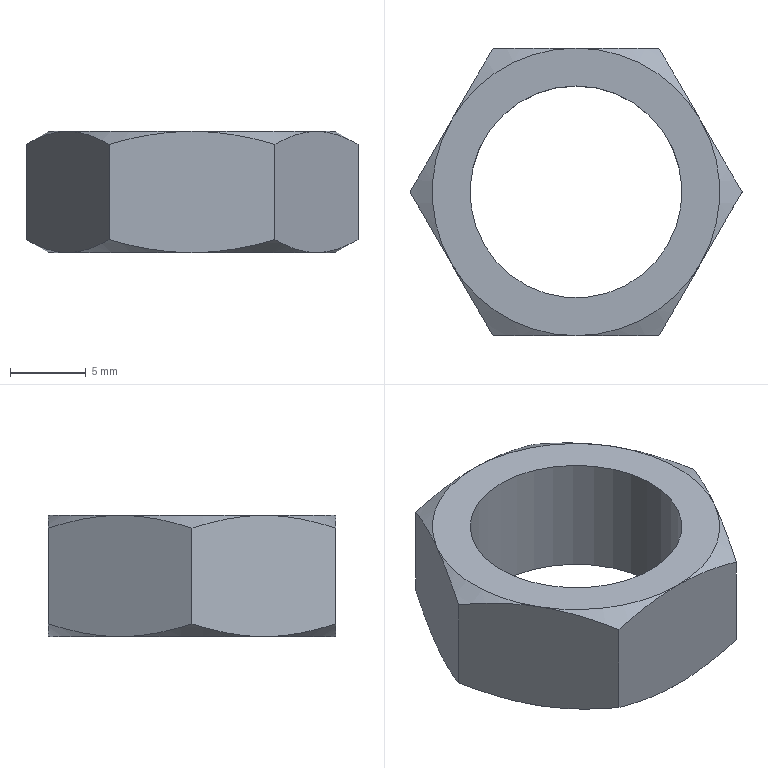Part | STEP file | 冲床-300配套压波_id646_x_t | 1 solid | 21 faces | box 21.939 x 19 x 8 mm | volume 1254 mm3 | cone 12 | plane 8 | cylinder 1 | commonest cylinder face diameters 14 x1
STEP:
#1=CARTESIAN_POINT('',(1810.485,9.5,205.151));
#2=VERTEX_POINT('',#1);
#3=CARTESIAN_POINT('',(1805.,9.5,206.));
#4=VERTEX_POINT('',#3);
#5=CARTESIAN_POINT('',(1810.485,9.5,205.151));
#6=CARTESIAN_POINT('',(1808.693,9.5,205.669));
#7=CARTESIAN_POINT('',(1806.872,9.5,206.));
#8=CARTESIAN_POINT('',(1805.,9.5,206.));
#9=B_SPLINE_CURVE_WITH_KNOTS('',3,(#5,#6,#7,#8),.UNSPECIFIED.,.F.,.F.,(4,4),(0.,1.),.UNSPECIFIED.);
#10=EDGE_CURVE('',#2,#4,#9,.T.);
#11=ORIENTED_EDGE('',*,*,#10,.F.);
#12=CARTESIAN_POINT('',(1810.485,9.5,198.849));
#13=VERTEX_POINT('',#12);
#14=CARTESIAN_POINT('',(1810.485,9.5,198.));
#15=DIRECTION('',(0.,0.,1.));
#16=VECTOR('',#15,1.);
#17=LINE('',#14,#16);
#18=EDGE_CURVE('',#13,#2,#17,.T.);
#19=ORIENTED_EDGE('',*,*,#18,.F.);
#20=CARTESIAN_POINT('',(1805.,9.5,198.));
#21=VERTEX_POINT('',#20);
#22=CARTESIAN_POINT('',(1805.,9.5,198.));
#23=CARTESIAN_POINT('',(1806.872,9.5,198.));
#24=CARTESIAN_POINT('',(1808.693,9.5,198.331));
#25=CARTESIAN_POINT('',(1810.485,9.5,198.849));
#26=B_SPLINE_CURVE_WITH_KNOTS('',3,(#22,#23,#24,#25),.UNSPECIFIED.,.F.,.F.,(4,4),(0.,1.),.UNSPECIFIED.);
#27=EDGE_CURVE('',#21,#13,#26,.T.);
#28=ORIENTED_EDGE('',*,*,#27,.F.);
#29=CARTESIAN_POINT('',(1799.515,9.5,198.849));
#30=VERTEX_POINT('',#29);
#31=CARTESIAN_POINT('',(1799.515,9.5,198.849));
#32=CARTESIAN_POINT('',(1801.307,9.5,198.331));
#33=CARTESIAN_POINT('',(1803.128,9.5,198.));
#34=CARTESIAN_POINT('',(1805.,9.5,198.));
#35=B_SPLINE_CURVE_WITH_KNOTS('',3,(#31,#32,#33,#34),.UNSPECIFIED.,.F.,.F.,(4,4),(0.,1.),.UNSPECIFIED.);
#36=EDGE_CURVE('',#30,#21,#35,.T.);
#37=ORIENTED_EDGE('',*,*,#36,.F.);
#38=CARTESIAN_POINT('',(1799.515,9.5,205.151));
#39=VERTEX_POINT('',#38);
#40=CARTESIAN_POINT('',(1799.515,9.5,198.));
#41=DIRECTION('',(0.,0.,1.));
#42=VECTOR('',#41,1.);
#43=LINE('',#40,#42);
#44=EDGE_CURVE('',#30,#39,#43,.T.);
#45=ORIENTED_EDGE('',*,*,#44,.T.);
#46=CARTESIAN_POINT('',(1805.,9.5,206.));
#47=CARTESIAN_POINT('',(1803.128,9.5,206.));
#48=CARTESIAN_POINT('',(1801.307,9.5,205.669));
#49=CARTESIAN_POINT('',(1799.515,9.5,205.151));
#50=B_SPLINE_CURVE_WITH_KNOTS('',3,(#46,#47,#48,#49),.UNSPECIFIED.,.F.,.F.,(4,4),(0.,1.),.UNSPECIFIED.);
#51=EDGE_CURVE('',#4,#39,#50,.T.);
#52=ORIENTED_EDGE('',*,*,#51,.F.);
#53=EDGE_LOOP('',(#11,#19,#28,#37,#45,#52));
#54=FACE_OUTER_BOUND('',#53,.T.);
#55=CARTESIAN_POINT('',(1799.515,9.5,198.));
#56=DIRECTION('',(0.,-1.,0.));
#57=DIRECTION('',(-1.,0.,0.));
#58=AXIS2_PLACEMENT_3D('',#55,#56,#57);
#59=PLANE('',#58);
#60=ADVANCED_FACE('',(#54),#59,.F.);
#61=CARTESIAN_POINT('',(1815.97,0.,205.151));
#62=VERTEX_POINT('',#61);
#63=CARTESIAN_POINT('',(1813.227,4.75,206.));
#64=VERTEX_POINT('',#63);
#65=CARTESIAN_POINT('',(1815.97,0.,205.151));
#66=CARTESIAN_POINT('',(1815.074,1.552,205.669));
#67=CARTESIAN_POINT('',(1814.163,3.129,206.));
#68=CARTESIAN_POINT('',(1813.227,4.75,206.));
#69=B_SPLINE_CURVE_WITH_KNOTS('',3,(#65,#66,#67,#68),.UNSPECIFIED.,.F.,.F.,(4,4),(0.,1.),.UNSPECIFIED.);
#70=EDGE_CURVE('',#62,#64,#69,.T.);
#71=ORIENTED_EDGE('',*,*,#70,.F.);
#72=CARTESIAN_POINT('',(1815.97,0.,198.849));
#73=VERTEX_POINT('',#72);
#74=CARTESIAN_POINT('',(1815.97,0.,198.));
#75=DIRECTION('',(0.,0.,1.));
#76=VECTOR('',#75,1.);
#77=LINE('',#74,#76);
#78=EDGE_CURVE('',#73,#62,#77,.T.);
#79=ORIENTED_EDGE('',*,*,#78,.F.);
#80=CARTESIAN_POINT('',(1813.227,4.75,198.));
#81=VERTEX_POINT('',#80);
#82=CARTESIAN_POINT('',(1813.227,4.75,198.));
#83=CARTESIAN_POINT('',(1814.163,3.129,198.));
#84=CARTESIAN_POINT('',(1815.074,1.552,198.331));
#85=CARTESIAN_POINT('',(1815.97,0.,198.849));
#86=B_SPLINE_CURVE_WITH_KNOTS('',3,(#82,#83,#84,#85),.UNSPECIFIED.,.F.,.F.,(4,4),(0.,1.),.UNSPECIFIED.);
#87=EDGE_CURVE('',#81,#73,#86,.T.);
#88=ORIENTED_EDGE('',*,*,#87,.F.);
#89=CARTESIAN_POINT('',(1810.485,9.5,198.849));
#90=CARTESIAN_POINT('',(1811.381,7.948,198.331));
#91=CARTESIAN_POINT('',(1812.291,6.371,198.));
#92=CARTESIAN_POINT('',(1813.227,4.75,198.));
#93=B_SPLINE_CURVE_WITH_KNOTS('',3,(#89,#90,#91,#92),.UNSPECIFIED.,.F.,.F.,(4,4),(0.,1.),.UNSPECIFIED.);
#94=EDGE_CURVE('',#13,#81,#93,.T.);
#95=ORIENTED_EDGE('',*,*,#94,.F.);
#96=ORIENTED_EDGE('',*,*,#18,.T.);
#97=CARTESIAN_POINT('',(1813.227,4.75,206.));
#98=CARTESIAN_POINT('',(1812.291,6.371,206.));
#99=CARTESIAN_POINT('',(1811.381,7.948,205.669));
#100=CARTESIAN_POINT('',(1810.485,9.5,205.151));
#101=B_SPLINE_CURVE_WITH_KNOTS('',3,(#97,#98,#99,#100),.UNSPECIFIED.,.F.,.F.,(4,4),(0.,1.),.UNSPECIFIED.);
#102=EDGE_CURVE('',#64,#2,#101,.T.);
#103=ORIENTED_EDGE('',*,*,#102,.F.);
#104=EDGE_LOOP('',(#71,#79,#88,#95,#96,#103));
#105=FACE_OUTER_BOUND('',#104,.T.);
#106=CARTESIAN_POINT('',(1810.485,9.5,198.));
#107=DIRECTION('',(-0.866,-0.5,0.));
#108=DIRECTION('',(-0.5,0.866,0.));
#109=AXIS2_PLACEMENT_3D('',#106,#107,#108);
#110=PLANE('',#109);
#111=ADVANCED_FACE('',(#105),#110,.F.);
#112=CARTESIAN_POINT('',(1810.485,-9.5,205.151));
#113=VERTEX_POINT('',#112);
#114=CARTESIAN_POINT('',(1813.227,-4.75,206.));
#115=VERTEX_POINT('',#114);
#116=CARTESIAN_POINT('',(1810.485,-9.5,205.151));
#117=CARTESIAN_POINT('',(1811.381,-7.948,205.669));
#118=CARTESIAN_POINT('',(1812.291,-6.371,206.));
#119=CARTESIAN_POINT('',(1813.227,-4.75,206.));
#120=B_SPLINE_CURVE_WITH_KNOTS('',3,(#116,#117,#118,#119),.UNSPECIFIED.,.F.,.F.,(4,4),(0.,1.),.UNSPECIFIED.);
#121=EDGE_CURVE('',#113,#115,#120,.T.);
#122=ORIENTED_EDGE('',*,*,#121,.F.);
#123=CARTESIAN_POINT('',(1810.485,-9.5,198.849));
#124=VERTEX_POINT('',#123);
#125=CARTESIAN_POINT('',(1810.485,-9.5,198.));
#126=DIRECTION('',(0.,0.,1.));
#127=VECTOR('',#126,1.);
#128=LINE('',#125,#127);
#129=EDGE_CURVE('',#124,#113,#128,.T.);
#130=ORIENTED_EDGE('',*,*,#129,.F.);
#131=CARTESIAN_POINT('',(1813.227,-4.75,198.));
#132=VERTEX_POINT('',#131);
#133=CARTESIAN_POINT('',(1813.227,-4.75,198.));
#134=CARTESIAN_POINT('',(1812.291,-6.371,198.));
#135=CARTESIAN_POINT('',(1811.381,-7.948,198.331));
#136=CARTESIAN_POINT('',(1810.485,-9.5,198.849));
#137=B_SPLINE_CURVE_WITH_KNOTS('',3,(#133,#134,#135,#136),.UNSPECIFIED.,.F.,.F.,(4,4),(0.,1.),.UNSPECIFIED.);
#138=EDGE_CURVE('',#132,#124,#137,.T.);
#139=ORIENTED_EDGE('',*,*,#138,.F.);
#140=CARTESIAN_POINT('',(1815.97,0.,198.849));
#141=CARTESIAN_POINT('',(1815.074,-1.552,198.331));
#142=CARTESIAN_POINT('',(1814.163,-3.129,198.));
#143=CARTESIAN_POINT('',(1813.227,-4.75,198.));
#144=B_SPLINE_CURVE_WITH_KNOTS('',3,(#140,#141,#142,#143),.UNSPECIFIED.,.F.,.F.,(4,4),(0.,1.),.UNSPECIFIED.);
#145=EDGE_CURVE('',#73,#132,#144,.T.);
#146=ORIENTED_EDGE('',*,*,#145,.F.);
#147=ORIENTED_EDGE('',*,*,#78,.T.);
#148=CARTESIAN_POINT('',(1813.227,-4.75,206.));
#149=CARTESIAN_POINT('',(1814.163,-3.129,206.));
#150=CARTESIAN_POINT('',(1815.074,-1.552,205.669));
#151=CARTESIAN_POINT('',(1815.97,0.,205.151));
#152=B_SPLINE_CURVE_WITH_KNOTS('',3,(#148,#149,#150,#151),.UNSPECIFIED.,.F.,.F.,(4,4),(0.,1.),.UNSPECIFIED.);
#153=EDGE_CURVE('',#115,#62,#152,.T.);
#154=ORIENTED_EDGE('',*,*,#153,.F.);
#155=EDGE_LOOP('',(#122,#130,#139,#146,#147,#154));
#156=FACE_OUTER_BOUND('',#155,.T.);
#157=CARTESIAN_POINT('',(1815.97,0.,198.));
#158=DIRECTION('',(-0.866,0.5,0.));
#159=DIRECTION('',(0.5,0.866,0.));
#160=AXIS2_PLACEMENT_3D('',#157,#158,#159);
#161=PLANE('',#160);
#162=ADVANCED_FACE('',(#156),#161,.F.);
#163=CARTESIAN_POINT('',(1799.515,-9.5,205.151));
#164=VERTEX_POINT('',#163);
#165=CARTESIAN_POINT('',(1805.,-9.5,206.));
#166=VERTEX_POINT('',#165);
#167=CARTESIAN_POINT('',(1799.515,-9.5,205.151));
#168=CARTESIAN_POINT('',(1801.307,-9.5,205.669));
#169=CARTESIAN_POINT('',(1803.128,-9.5,206.));
#170=CARTESIAN_POINT('',(1805.,-9.5,206.));
#171=B_SPLINE_CURVE_WITH_KNOTS('',3,(#167,#168,#169,#170),.UNSPECIFIED.,.F.,.F.,(4,4),(0.,1.),.UNSPECIFIED.);
#172=EDGE_CURVE('',#164,#166,#171,.T.);
#173=ORIENTED_EDGE('',*,*,#172,.F.);
#174=CARTESIAN_POINT('',(1799.515,-9.5,198.849));
#175=VERTEX_POINT('',#174);
#176=CARTESIAN_POINT('',(1799.515,-9.5,198.));
#177=DIRECTION('',(0.,0.,1.));
#178=VECTOR('',#177,1.);
#179=LINE('',#176,#178);
#180=EDGE_CURVE('',#175,#164,#179,.T.);
#181=ORIENTED_EDGE('',*,*,#180,.F.);
#182=CARTESIAN_POINT('',(1805.,-9.5,198.));
#183=VERTEX_POINT('',#182);
#184=CARTESIAN_POINT('',(1805.,-9.5,198.));
#185=CARTESIAN_POINT('',(1803.128,-9.5,198.));
#186=CARTESIAN_POINT('',(1801.307,-9.5,198.331));
#187=CARTESIAN_POINT('',(1799.515,-9.5,198.849));
#188=B_SPLINE_CURVE_WITH_KNOTS('',3,(#184,#185,#186,#187),.UNSPECIFIED.,.F.,.F.,(4,4),(0.,1.),.UNSPECIFIED.);
#189=EDGE_CURVE('',#183,#175,#188,.T.);
#190=ORIENTED_EDGE('',*,*,#189,.F.);
#191=CARTESIAN_POINT('',(1810.485,-9.5,198.849));
#192=CARTESIAN_POINT('',(1808.693,-9.5,198.331));
#193=CARTESIAN_POINT('',(1806.872,-9.5,198.));
#194=CARTESIAN_POINT('',(1805.,-9.5,198.));
#195=B_SPLINE_CURVE_WITH_KNOTS('',3,(#191,#192,#193,#194),.UNSPECIFIED.,.F.,.F.,(4,4),(0.,1.),.UNSPECIFIED.);
#196=EDGE_CURVE('',#124,#183,#195,.T.);
#197=ORIENTED_EDGE('',*,*,#196,.F.);
#198=ORIENTED_EDGE('',*,*,#129,.T.);
#199=CARTESIAN_POINT('',(1805.,-9.5,206.));
#200=CARTESIAN_POINT('',(1806.872,-9.5,206.));
#201=CARTESIAN_POINT('',(1808.693,-9.5,205.669));
#202=CARTESIAN_POINT('',(1810.485,-9.5,205.151));
#203=B_SPLINE_CURVE_WITH_KNOTS('',3,(#199,#200,#201,#202),.UNSPECIFIED.,.F.,.F.,(4,4),(0.,1.),.UNSPECIFIED.);
#204=EDGE_CURVE('',#166,#113,#203,.T.);
#205=ORIENTED_EDGE('',*,*,#204,.F.);
#206=EDGE_LOOP('',(#173,#181,#190,#197,#198,#205));
#207=FACE_OUTER_BOUND('',#206,.T.);
#208=CARTESIAN_POINT('',(1810.485,-9.5,198.));
#209=DIRECTION('',(0.,1.,0.));
#210=DIRECTION('',(1.,0.,0.));
#211=AXIS2_PLACEMENT_3D('',#208,#209,#210);
#212=PLANE('',#211);
#213=ADVANCED_FACE('',(#207),#212,.F.);
#214=CARTESIAN_POINT('',(1794.03,0.,205.151));
#215=VERTEX_POINT('',#214);
#216=CARTESIAN_POINT('',(1796.773,-4.75,206.));
#217=VERTEX_POINT('',#216);
#218=CARTESIAN_POINT('',(1794.03,0.,205.151));
#219=CARTESIAN_POINT('',(1794.926,-1.552,205.669));
#220=CARTESIAN_POINT('',(1795.837,-3.129,206.));
#221=CARTESIAN_POINT('',(1796.773,-4.75,206.));
#222=B_SPLINE_CURVE_WITH_KNOTS('',3,(#218,#219,#220,#221),.UNSPECIFIED.,.F.,.F.,(4,4),(0.,1.),.UNSPECIFIED.);
#223=EDGE_CURVE('',#215,#217,#222,.T.);
#224=ORIENTED_EDGE('',*,*,#223,.F.);
#225=CARTESIAN_POINT('',(1794.03,0.,198.849));
#226=VERTEX_POINT('',#225);
#227=CARTESIAN_POINT('',(1794.03,0.,198.));
#228=DIRECTION('',(0.,0.,1.));
#229=VECTOR('',#228,1.);
#230=LINE('',#227,#229);
#231=EDGE_CURVE('',#226,#215,#230,.T.);
#232=ORIENTED_EDGE('',*,*,#231,.F.);
#233=CARTESIAN_POINT('',(1796.773,-4.75,198.));
#234=VERTEX_POINT('',#233);
#235=CARTESIAN_POINT('',(1796.773,-4.75,198.));
#236=CARTESIAN_POINT('',(1795.837,-3.129,198.));
#237=CARTESIAN_POINT('',(1794.926,-1.552,198.331));
#238=CARTESIAN_POINT('',(1794.03,0.,198.849));
#239=B_SPLINE_CURVE_WITH_KNOTS('',3,(#235,#236,#237,#238),.UNSPECIFIED.,.F.,.F.,(4,4),(0.,1.),.UNSPECIFIED.);
#240=EDGE_CURVE('',#234,#226,#239,.T.);
#241=ORIENTED_EDGE('',*,*,#240,.F.);
#242=CARTESIAN_POINT('',(1799.515,-9.5,198.849));
#243=CARTESIAN_POINT('',(1798.619,-7.948,198.331));
#244=CARTESIAN_POINT('',(1797.709,-6.371,198.));
#245=CARTESIAN_POINT('',(1796.773,-4.75,198.));
#246=B_SPLINE_CURVE_WITH_KNOTS('',3,(#242,#243,#244,#245),.UNSPECIFIED.,.F.,.F.,(4,4),(0.,1.),.UNSPECIFIED.);
#247=EDGE_CURVE('',#175,#234,#246,.T.);
#248=ORIENTED_EDGE('',*,*,#247,.F.);
#249=ORIENTED_EDGE('',*,*,#180,.T.);
#250=CARTESIAN_POINT('',(1796.773,-4.75,206.));
#251=CARTESIAN_POINT('',(1797.709,-6.371,206.));
#252=CARTESIAN_POINT('',(1798.619,-7.948,205.669));
#253=CARTESIAN_POINT('',(1799.515,-9.5,205.151));
#254=B_SPLINE_CURVE_WITH_KNOTS('',3,(#250,#251,#252,#253),.UNSPECIFIED.,.F.,.F.,(4,4),(0.,1.),.UNSPECIFIED.);
#255=EDGE_CURVE('',#217,#164,#254,.T.);
#256=ORIENTED_EDGE('',*,*,#255,.F.);
#257=EDGE_LOOP('',(#224,#232,#241,#248,#249,#256));
#258=FACE_OUTER_BOUND('',#257,.T.);
#259=CARTESIAN_POINT('',(1799.515,-9.5,198.));
#260=DIRECTION('',(0.866,0.5,0.));
#261=DIRECTION('',(0.5,-0.866,0.));
#262=AXIS2_PLACEMENT_3D('',#259,#260,#261);
#263=PLANE('',#262);
#264=ADVANCED_FACE('',(#258),#263,.F.);
#265=CARTESIAN_POINT('',(1796.773,4.75,206.));
#266=VERTEX_POINT('',#265);
#267=CARTESIAN_POINT('',(1799.515,9.5,205.151));
#268=CARTESIAN_POINT('',(1798.619,7.948,205.669));
#269=CARTESIAN_POINT('',(1797.709,6.371,206.));
#270=CARTESIAN_POINT('',(1796.773,4.75,206.));
#271=B_SPLINE_CURVE_WITH_KNOTS('',3,(#267,#268,#269,#270),.UNSPECIFIED.,.F.,.F.,(4,4),(0.,1.),.UNSPECIFIED.);
#272=EDGE_CURVE('',#39,#266,#271,.T.);
#273=ORIENTED_EDGE('',*,*,#272,.F.);
#274=ORIENTED_EDGE('',*,*,#44,.F.);
#275=CARTESIAN_POINT('',(1796.773,4.75,198.));
#276=VERTEX_POINT('',#275);
#277=CARTESIAN_POINT('',(1796.773,4.75,198.));
#278=CARTESIAN_POINT('',(1797.709,6.371,198.));
#279=CARTESIAN_POINT('',(1798.619,7.948,198.331));
#280=CARTESIAN_POINT('',(1799.515,9.5,198.849));
#281=B_SPLINE_CURVE_WITH_KNOTS('',3,(#277,#278,#279,#280),.UNSPECIFIED.,.F.,.F.,(4,4),(0.,1.),.UNSPECIFIED.);
#282=EDGE_CURVE('',#276,#30,#281,.T.);
#283=ORIENTED_EDGE('',*,*,#282,.F.);
#284=CARTESIAN_POINT('',(1794.03,0.,198.849));
#285=CARTESIAN_POINT('',(1794.926,1.552,198.331));
#286=CARTESIAN_POINT('',(1795.837,3.129,198.));
#287=CARTESIAN_POINT('',(1796.773,4.75,198.));
#288=B_SPLINE_CURVE_WITH_KNOTS('',3,(#284,#285,#286,#287),.UNSPECIFIED.,.F.,.F.,(4,4),(0.,1.),.UNSPECIFIED.);
#289=EDGE_CURVE('',#226,#276,#288,.T.);
#290=ORIENTED_EDGE('',*,*,#289,.F.);
#291=ORIENTED_EDGE('',*,*,#231,.T.);
#292=CARTESIAN_POINT('',(1796.773,4.75,206.));
#293=CARTESIAN_POINT('',(1795.837,3.129,206.));
#294=CARTESIAN_POINT('',(1794.926,1.552,205.669));
#295=CARTESIAN_POINT('',(1794.03,0.,205.151));
#296=B_SPLINE_CURVE_WITH_KNOTS('',3,(#292,#293,#294,#295),.UNSPECIFIED.,.F.,.F.,(4,4),(0.,1.),.UNSPECIFIED.);
#297=EDGE_CURVE('',#266,#215,#296,.T.);
#298=ORIENTED_EDGE('',*,*,#297,.F.);
#299=EDGE_LOOP('',(#273,#274,#283,#290,#291,#298));
#300=FACE_OUTER_BOUND('',#299,.T.);
#301=CARTESIAN_POINT('',(1794.03,0.,198.));
#302=DIRECTION('',(0.866,-0.5,0.));
#303=DIRECTION('',(-0.5,-0.866,0.));
#304=AXIS2_PLACEMENT_3D('',#301,#302,#303);
#305=PLANE('',#304);
#306=ADVANCED_FACE('',(#300),#305,.F.);
#307=CARTESIAN_POINT('',(1805.,7.,206.));
#308=VERTEX_POINT('',#307);
#309=CARTESIAN_POINT('',(1805.,0.,206.));
#310=DIRECTION('',(0.,0.,1.));
#311=DIRECTION('',(0.,1.,0.));
#312=AXIS2_PLACEMENT_3D('',#309,#310,#311);
#313=CIRCLE('',#312,7.);
#314=EDGE_CURVE('',#308,#308,#313,.T.);
#315=ORIENTED_EDGE('',*,*,#314,.F.);
#316=EDGE_LOOP('',(#315));
#317=FACE_BOUND('',#316,.T.);
#318=CARTESIAN_POINT('',(1805.,0.,206.));
#319=DIRECTION('',(0.,0.,-1.));
#320=DIRECTION('',(-1.,0.,0.));
#321=AXIS2_PLACEMENT_3D('',#318,#319,#320);
#322=CIRCLE('',#321,9.5);
#323=EDGE_CURVE('',#266,#4,#322,.T.);
#324=ORIENTED_EDGE('',*,*,#323,.F.);
#325=CARTESIAN_POINT('',(1805.,0.,206.));
#326=DIRECTION('',(0.,0.,-1.));
#327=DIRECTION('',(-1.,0.,0.));
#328=AXIS2_PLACEMENT_3D('',#325,#326,#327);
#329=CIRCLE('',#328,9.5);
#330=EDGE_CURVE('',#217,#266,#329,.T.);
#331=ORIENTED_EDGE('',*,*,#330,.F.);
#332=CARTESIAN_POINT('',(1805.,0.,206.));
#333=DIRECTION('',(0.,0.,-1.));
#334=DIRECTION('',(-1.,0.,0.));
#335=AXIS2_PLACEMENT_3D('',#332,#333,#334);
#336=CIRCLE('',#335,9.5);
#337=EDGE_CURVE('',#166,#217,#336,.T.);
#338=ORIENTED_EDGE('',*,*,#337,.F.);
#339=CARTESIAN_POINT('',(1805.,0.,206.));
#340=DIRECTION('',(0.,0.,1.));
#341=DIRECTION('',(1.,0.,0.));
#342=AXIS2_PLACEMENT_3D('',#339,#340,#341);
#343=CIRCLE('',#342,9.5);
#344=EDGE_CURVE('',#166,#115,#343,.T.);
#345=ORIENTED_EDGE('',*,*,#344,.T.);
#346=CARTESIAN_POINT('',(1805.,0.,206.));
#347=DIRECTION('',(0.,0.,-1.));
#348=DIRECTION('',(-1.,0.,0.));
#349=AXIS2_PLACEMENT_3D('',#346,#347,#348);
#350=CIRCLE('',#349,9.5);
#351=EDGE_CURVE('',#64,#115,#350,.T.);
#352=ORIENTED_EDGE('',*,*,#351,.F.);
#353=CARTESIAN_POINT('',(1805.,0.,206.));
#354=DIRECTION('',(0.,0.,-1.));
#355=DIRECTION('',(-1.,0.,0.));
#356=AXIS2_PLACEMENT_3D('',#353,#354,#355);
#357=CIRCLE('',#356,9.5);
#358=EDGE_CURVE('',#4,#64,#357,.T.);
#359=ORIENTED_EDGE('',*,*,#358,.F.);
#360=EDGE_LOOP('',(#324,#331,#338,#345,#352,#359));
#361=FACE_BOUND('',#360,.T.);
#362=CARTESIAN_POINT('',(1805.,0.,206.));
#363=DIRECTION('',(0.,0.,-1.));
#364=DIRECTION('',(1.,0.,0.));
#365=AXIS2_PLACEMENT_3D('',#362,#363,#364);
#366=PLANE('',#365);
#367=ADVANCED_FACE('',(#317,#361),#366,.F.);
#368=CARTESIAN_POINT('',(1805.,7.,198.));
#369=VERTEX_POINT('',#368);
#370=CARTESIAN_POINT('',(1805.,0.,198.));
#371=DIRECTION('',(0.,0.,1.));
#372=DIRECTION('',(0.,1.,0.));
#373=AXIS2_PLACEMENT_3D('',#370,#371,#372);
#374=CIRCLE('',#373,7.);
#375=EDGE_CURVE('',#369,#369,#374,.T.);
#376=ORIENTED_EDGE('',*,*,#375,.T.);
#377=EDGE_LOOP('',(#376));
#378=FACE_BOUND('',#377,.T.);
#379=CARTESIAN_POINT('',(1805.,0.,198.));
#380=DIRECTION('',(0.,0.,-1.));
#381=DIRECTION('',(-1.,0.,0.));
#382=AXIS2_PLACEMENT_3D('',#379,#380,#381);
#383=CIRCLE('',#382,9.5);
#384=EDGE_CURVE('',#234,#276,#383,.T.);
#385=ORIENTED_EDGE('',*,*,#384,.T.);
#386=CARTESIAN_POINT('',(1805.,0.,198.));
#387=DIRECTION('',(0.,0.,-1.));
#388=DIRECTION('',(-1.,0.,0.));
#389=AXIS2_PLACEMENT_3D('',#386,#387,#388);
#390=CIRCLE('',#389,9.5);
#391=EDGE_CURVE('',#276,#21,#390,.T.);
#392=ORIENTED_EDGE('',*,*,#391,.T.);
#393=CARTESIAN_POINT('',(1805.,0.,198.));
#394=DIRECTION('',(0.,0.,-1.));
#395=DIRECTION('',(-1.,0.,0.));
#396=AXIS2_PLACEMENT_3D('',#393,#394,#395);
#397=CIRCLE('',#396,9.5);
#398=EDGE_CURVE('',#21,#81,#397,.T.);
#399=ORIENTED_EDGE('',*,*,#398,.T.);
#400=CARTESIAN_POINT('',(1805.,0.,198.));
#401=DIRECTION('',(0.,0.,-1.));
#402=DIRECTION('',(-1.,0.,0.));
#403=AXIS2_PLACEMENT_3D('',#400,#401,#402);
#404=CIRCLE('',#403,9.5);
#405=EDGE_CURVE('',#81,#132,#404,.T.);
#406=ORIENTED_EDGE('',*,*,#405,.T.);
#407=CARTESIAN_POINT('',(1805.,0.,198.));
#408=DIRECTION('',(0.,0.,1.));
#409=DIRECTION('',(1.,0.,0.));
#410=AXIS2_PLACEMENT_3D('',#407,#408,#409);
#411=CIRCLE('',#410,9.5);
#412=EDGE_CURVE('',#183,#132,#411,.T.);
#413=ORIENTED_EDGE('',*,*,#412,.F.);
#414=CARTESIAN_POINT('',(1805.,0.,198.));
#415=DIRECTION('',(0.,0.,-1.));
#416=DIRECTION('',(-1.,0.,0.));
#417=AXIS2_PLACEMENT_3D('',#414,#415,#416);
#418=CIRCLE('',#417,9.5);
#419=EDGE_CURVE('',#183,#234,#418,.T.);
#420=ORIENTED_EDGE('',*,*,#419,.T.);
#421=EDGE_LOOP('',(#385,#392,#399,#406,#413,#420));
#422=FACE_BOUND('',#421,.T.);
#423=CARTESIAN_POINT('',(1805.,0.,198.));
#424=DIRECTION('',(0.,0.,-1.));
#425=DIRECTION('',(1.,0.,0.));
#426=AXIS2_PLACEMENT_3D('',#423,#424,#425);
#427=PLANE('',#426);
#428=ADVANCED_FACE('',(#378,#422),#427,.T.);
#429=ORIENTED_EDGE('',*,*,#375,.F.);
#430=EDGE_LOOP('',(#429));
#431=FACE_BOUND('',#430,.T.);
#432=ORIENTED_EDGE('',*,*,#314,.T.);
#433=EDGE_LOOP('',(#432));
#434=FACE_BOUND('',#433,.T.);
#435=CARTESIAN_POINT('',(1805.,0.,198.));
#436=DIRECTION('',(0.,0.,1.));
#437=DIRECTION('',(-1.,0.,0.));
#438=AXIS2_PLACEMENT_3D('',#435,#436,#437);
#439=CYLINDRICAL_SURFACE('',#438,7.);
#440=ADVANCED_FACE('',(#431,#434),#439,.F.);
#441=ORIENTED_EDGE('',*,*,#240,.T.);
#442=ORIENTED_EDGE('',*,*,#289,.T.);
#443=ORIENTED_EDGE('',*,*,#384,.F.);
#444=EDGE_LOOP('',(#441,#442,#443));
#445=FACE_OUTER_BOUND('',#444,.T.);
#446=CARTESIAN_POINT('',(1805.,0.,200.5));
#447=DIRECTION('',(0.,0.,1.));
#448=DIRECTION('',(-1.,0.,0.));
#449=AXIS2_PLACEMENT_3D('',#446,#447,#448);
#450=CONICAL_SURFACE('',#449,13.83,60.);
#451=ADVANCED_FACE('',(#445),#450,.T.);
#452=ORIENTED_EDGE('',*,*,#189,.T.);
#453=ORIENTED_EDGE('',*,*,#247,.T.);
#454=ORIENTED_EDGE('',*,*,#419,.F.);
#455=EDGE_LOOP('',(#452,#453,#454));
#456=FACE_OUTER_BOUND('',#455,.T.);
#457=CARTESIAN_POINT('',(1805.,0.,200.5));
#458=DIRECTION('',(0.,0.,1.));
#459=DIRECTION('',(-1.,0.,0.));
#460=AXIS2_PLACEMENT_3D('',#457,#458,#459);
#461=CONICAL_SURFACE('',#460,13.83,60.);
#462=ADVANCED_FACE('',(#456),#461,.T.);
#463=ORIENTED_EDGE('',*,*,#138,.T.);
#464=ORIENTED_EDGE('',*,*,#196,.T.);
#465=ORIENTED_EDGE('',*,*,#412,.T.);
#466=EDGE_LOOP('',(#463,#464,#465));
#467=FACE_OUTER_BOUND('',#466,.T.);
#468=CARTESIAN_POINT('',(1805.,0.,200.5));
#469=DIRECTION('',(0.,0.,1.));
#470=DIRECTION('',(-1.,0.,0.));
#471=AXIS2_PLACEMENT_3D('',#468,#469,#470);
#472=CONICAL_SURFACE('',#471,13.83,60.);
#473=ADVANCED_FACE('',(#467),#472,.T.);
#474=ORIENTED_EDGE('',*,*,#87,.T.);
#475=ORIENTED_EDGE('',*,*,#145,.T.);
#476=ORIENTED_EDGE('',*,*,#405,.F.);
#477=EDGE_LOOP('',(#474,#475,#476));
#478=FACE_OUTER_BOUND('',#477,.T.);
#479=CARTESIAN_POINT('',(1805.,0.,200.5));
#480=DIRECTION('',(0.,0.,1.));
#481=DIRECTION('',(-1.,0.,0.));
#482=AXIS2_PLACEMENT_3D('',#479,#480,#481);
#483=CONICAL_SURFACE('',#482,13.83,60.);
#484=ADVANCED_FACE('',(#478),#483,.T.);
#485=ORIENTED_EDGE('',*,*,#27,.T.);
#486=ORIENTED_EDGE('',*,*,#94,.T.);
#487=ORIENTED_EDGE('',*,*,#398,.F.);
#488=EDGE_LOOP('',(#485,#486,#487));
#489=FACE_OUTER_BOUND('',#488,.T.);
#490=CARTESIAN_POINT('',(1805.,0.,200.5));
#491=DIRECTION('',(0.,0.,1.));
#492=DIRECTION('',(-1.,0.,0.));
#493=AXIS2_PLACEMENT_3D('',#490,#491,#492);
#494=CONICAL_SURFACE('',#493,13.83,60.);
#495=ADVANCED_FACE('',(#489),#494,.T.);
#496=ORIENTED_EDGE('',*,*,#36,.T.);
#497=ORIENTED_EDGE('',*,*,#391,.F.);
#498=ORIENTED_EDGE('',*,*,#282,.T.);
#499=EDGE_LOOP('',(#496,#497,#498));
#500=FACE_OUTER_BOUND('',#499,.T.);
#501=CARTESIAN_POINT('',(1805.,0.,200.5));
#502=DIRECTION('',(0.,0.,1.));
#503=DIRECTION('',(-1.,0.,0.));
#504=AXIS2_PLACEMENT_3D('',#501,#502,#503);
#505=CONICAL_SURFACE('',#504,13.83,60.);
#506=ADVANCED_FACE('',(#500),#505,.T.);
#507=ORIENTED_EDGE('',*,*,#223,.T.);
#508=ORIENTED_EDGE('',*,*,#330,.T.);
#509=ORIENTED_EDGE('',*,*,#297,.T.);
#510=EDGE_LOOP('',(#507,#508,#509));
#511=FACE_OUTER_BOUND('',#510,.T.);
#512=CARTESIAN_POINT('',(1805.,0.,206.));
#513=DIRECTION('',(0.,0.,-1.));
#514=DIRECTION('',(1.,0.,0.));
#515=AXIS2_PLACEMENT_3D('',#512,#513,#514);
#516=CONICAL_SURFACE('',#515,9.5,60.);
#517=ADVANCED_FACE('',(#511),#516,.T.);
#518=ORIENTED_EDGE('',*,*,#172,.T.);
#519=ORIENTED_EDGE('',*,*,#337,.T.);
#520=ORIENTED_EDGE('',*,*,#255,.T.);
#521=EDGE_LOOP('',(#518,#519,#520));
#522=FACE_OUTER_BOUND('',#521,.T.);
#523=CARTESIAN_POINT('',(1805.,0.,206.));
#524=DIRECTION('',(0.,0.,-1.));
#525=DIRECTION('',(1.,0.,0.));
#526=AXIS2_PLACEMENT_3D('',#523,#524,#525);
#527=CONICAL_SURFACE('',#526,9.5,60.);
#528=ADVANCED_FACE('',(#522),#527,.T.);
#529=ORIENTED_EDGE('',*,*,#121,.T.);
#530=ORIENTED_EDGE('',*,*,#344,.F.);
#531=ORIENTED_EDGE('',*,*,#204,.T.);
#532=EDGE_LOOP('',(#529,#530,#531));
#533=FACE_OUTER_BOUND('',#532,.T.);
#534=CARTESIAN_POINT('',(1805.,0.,206.));
#535=DIRECTION('',(0.,0.,-1.));
#536=DIRECTION('',(1.,0.,0.));
#537=AXIS2_PLACEMENT_3D('',#534,#535,#536);
#538=CONICAL_SURFACE('',#537,9.5,60.);
#539=ADVANCED_FACE('',(#533),#538,.T.);
#540=ORIENTED_EDGE('',*,*,#153,.T.);
#541=ORIENTED_EDGE('',*,*,#70,.T.);
#542=ORIENTED_EDGE('',*,*,#351,.T.);
#543=EDGE_LOOP('',(#540,#541,#542));
#544=FACE_OUTER_BOUND('',#543,.T.);
#545=CARTESIAN_POINT('',(1805.,0.,206.));
#546=DIRECTION('',(0.,0.,-1.));
#547=DIRECTION('',(1.,0.,0.));
#548=AXIS2_PLACEMENT_3D('',#545,#546,#547);
#549=CONICAL_SURFACE('',#548,9.5,60.);
#550=ADVANCED_FACE('',(#544),#549,.T.);
#551=ORIENTED_EDGE('',*,*,#102,.T.);
#552=ORIENTED_EDGE('',*,*,#10,.T.);
#553=ORIENTED_EDGE('',*,*,#358,.T.);
#554=EDGE_LOOP('',(#551,#552,#553));
#555=FACE_OUTER_BOUND('',#554,.T.);
#556=CARTESIAN_POINT('',(1805.,0.,206.));
#557=DIRECTION('',(0.,0.,-1.));
#558=DIRECTION('',(1.,0.,0.));
#559=AXIS2_PLACEMENT_3D('',#556,#557,#558);
#560=CONICAL_SURFACE('',#559,9.5,60.);
#561=ADVANCED_FACE('',(#555),#560,.T.);
#562=ORIENTED_EDGE('',*,*,#51,.T.);
#563=ORIENTED_EDGE('',*,*,#272,.T.);
#564=ORIENTED_EDGE('',*,*,#323,.T.);
#565=EDGE_LOOP('',(#562,#563,#564));
#566=FACE_OUTER_BOUND('',#565,.T.);
#567=CARTESIAN_POINT('',(1805.,0.,206.));
#568=DIRECTION('',(0.,0.,-1.));
#569=DIRECTION('',(1.,0.,0.));
#570=AXIS2_PLACEMENT_3D('',#567,#568,#569);
#571=CONICAL_SURFACE('',#570,9.5,60.);
#572=ADVANCED_FACE('',(#566),#571,.T.);
#573=CLOSED_SHELL('',(#60,#111,#162,#213,#264,#306,#367,#428,#440,#451,#462,#473,#484,#495,#506,#517,#528,#539,#550,#561,#572));
#574=MANIFOLD_SOLID_BREP('',#573);
#575=(LENGTH_UNIT()NAMED_UNIT(*)SI_UNIT(.MILLI.,.METRE.));
#576=UNCERTAINTY_MEASURE_WITH_UNIT(LENGTH_MEASURE(0.0508),#575,'','');
#577=(NAMED_UNIT(*)PLANE_ANGLE_UNIT()SI_UNIT($,.RADIAN.));
#578=PLANE_ANGLE_MEASURE_WITH_UNIT(PLANE_ANGLE_MEASURE(0.01745),#577);
#579=DIMENSIONAL_EXPONENTS(0.,0.,0.,0.,0.,0.,0.);
#580=(CONVERSION_BASED_UNIT('DEGREE',#578)NAMED_UNIT(#579)PLANE_ANGLE_UNIT());
#581=(NAMED_UNIT(*)SI_UNIT($,.STERADIAN.)SOLID_ANGLE_UNIT());
#582=(GEOMETRIC_REPRESENTATION_CONTEXT(3)GLOBAL_UNCERTAINTY_ASSIGNED_CONTEXT((#576))GLOBAL_UNIT_ASSIGNED_CONTEXT((#575,#580,#581))REPRESENTATION_CONTEXT('',''));
#583=ADVANCED_BREP_SHAPE_REPRESENTATION('',(#574),#582);